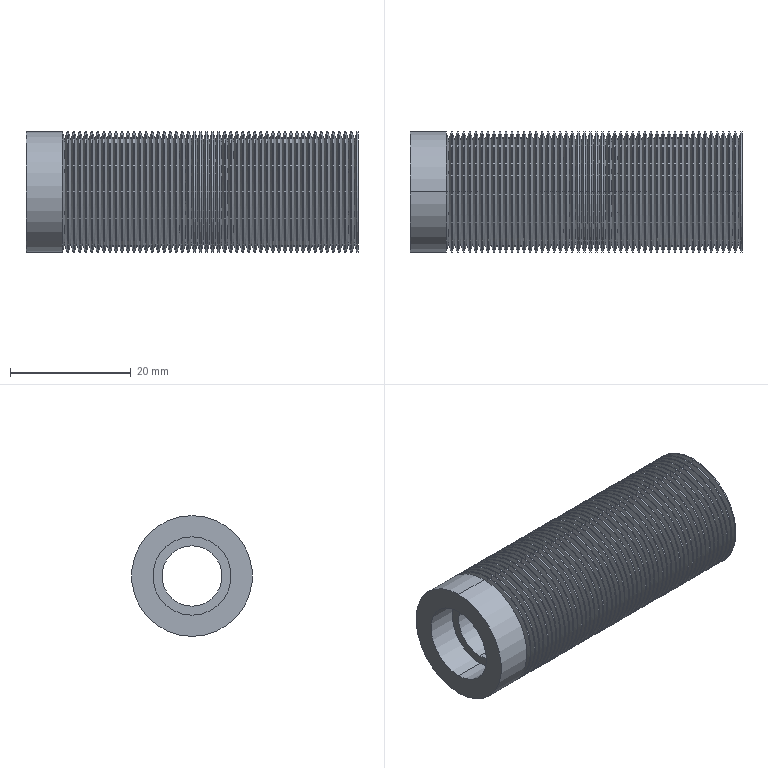Part | SolidWorks | features Revolution 1 | 1 solid | 306 faces | box 55 x 20 x 20 mm | volume 10654 mm3 | cone 196 | cylinder 106 | plane 4 | commonest cylinder face diameters 20 x100 13 x4 10 x2